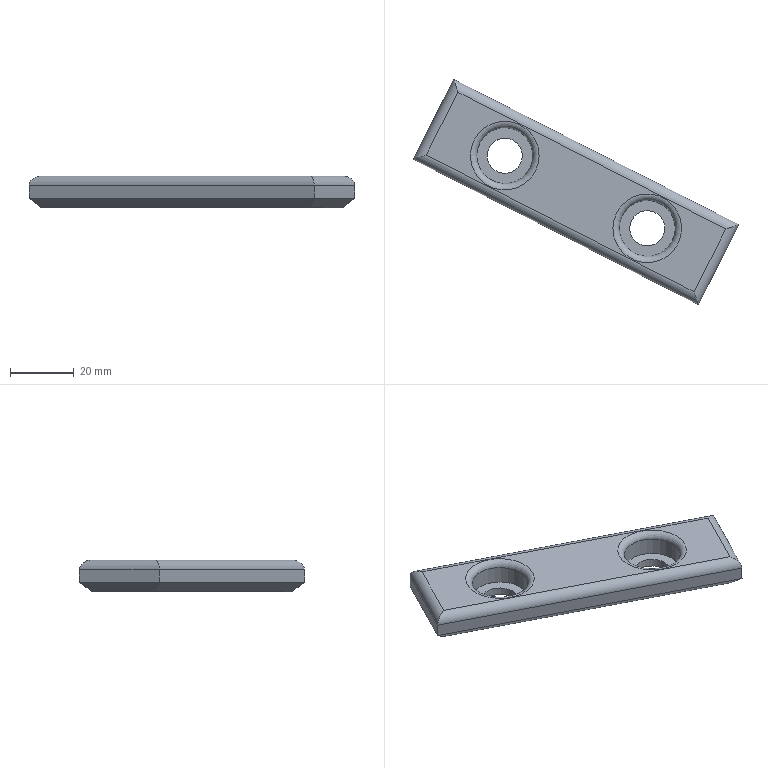Part | STEP file | gslz 2016.10.28-13_id1810_x_t | 1 solid | 22 faces | box 101.812 x 70.347 x 10 mm | volume 22218 mm3 | plane 12 | cylinder 8 | torus 2 | commonest cylinder face diameters 6 x4 11 x2 17.5 x2